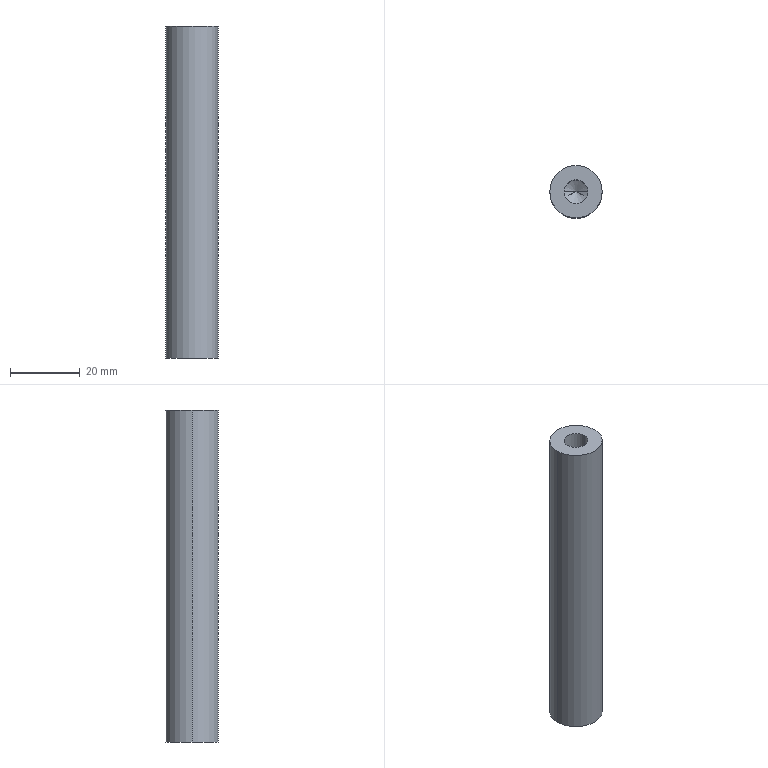Part | STEP file | Cuon T phu H01_10_1 | 1 solid | 8 faces | box 15 x 15 x 95 mm | volume 16046 mm3 | cylinder 4 | cone 2 | plane 2 | commonest cylinder face diameters 6.8 x2 15 x2
STEP:
#1=CARTESIAN_POINT('',(0.,0.,0.));
#2=DIRECTION('',(0.,0.,1.));
#3=DIRECTION('',(1.,0.,0.));
#4=AXIS2_PLACEMENT_3D('',#1,#2,#3);
#5=CARTESIAN_POINT('',(3.4,0.,27.75));
#6=VERTEX_POINT('',#5);
#7=CARTESIAN_POINT('',(3.4,0.,47.5));
#8=VERTEX_POINT('',#7);
#9=CARTESIAN_POINT('',(3.4,0.,47.5));
#10=DIRECTION('',(0.,0.,1.));
#11=VECTOR('',#10,1.);
#12=LINE('',#9,#11);
#13=CARTESIAN_POINT('',(0.,0.,47.5));
#14=DIRECTION('',(0.,0.,1.));
#15=DIRECTION('',(1.,0.,0.));
#16=AXIS2_PLACEMENT_3D('',#13,#14,#15);
#17=CYLINDRICAL_SURFACE('',#16,3.4);
#18=CARTESIAN_POINT('',(6.283,0.));
#19=DIRECTION('',(0.,1.));
#20=VECTOR('',#19,1.);
#21=LINE('',#18,#20);
#22=(GEOMETRIC_REPRESENTATION_CONTEXT(2)PARAMETRIC_REPRESENTATION_CONTEXT()REPRESENTATION_CONTEXT('',''));
#23=DEFINITIONAL_REPRESENTATION('',(#21),#22);
#24=PCURVE('',#17,#23);
#25=CARTESIAN_POINT('',(0.,0.,47.5));
#26=DIRECTION('',(0.,0.,1.));
#27=DIRECTION('',(1.,0.,0.));
#28=AXIS2_PLACEMENT_3D('',#25,#26,#27);
#29=CYLINDRICAL_SURFACE('',#28,3.4);
#30=CARTESIAN_POINT('',(0.,0.));
#31=DIRECTION('',(0.,1.));
#32=VECTOR('',#31,1.);
#33=LINE('',#30,#32);
#34=(GEOMETRIC_REPRESENTATION_CONTEXT(2)PARAMETRIC_REPRESENTATION_CONTEXT()REPRESENTATION_CONTEXT('',''));
#35=DEFINITIONAL_REPRESENTATION('',(#33),#34);
#36=PCURVE('',#29,#35);
#37=SURFACE_CURVE('',#12,(#24,#36),.PCURVE_S1.);
#38=EDGE_CURVE('',#6,#8,#37,.T.);
#39=ORIENTED_EDGE('',*,*,#38,.T.);
#40=CARTESIAN_POINT('',(-3.4,0.,47.5));
#41=VERTEX_POINT('',#40);
#42=CARTESIAN_POINT('',(0.,0.,47.5));
#43=DIRECTION('',(0.,0.,1.));
#44=DIRECTION('',(1.,0.,0.));
#45=AXIS2_PLACEMENT_3D('',#42,#43,#44);
#46=CIRCLE('',#45,3.4);
#47=CARTESIAN_POINT('',(0.,0.));
#48=DIRECTION('',(1.,0.));
#49=VECTOR('',#48,1.);
#50=LINE('',#47,#49);
#51=(GEOMETRIC_REPRESENTATION_CONTEXT(2)PARAMETRIC_REPRESENTATION_CONTEXT()REPRESENTATION_CONTEXT('',''));
#52=DEFINITIONAL_REPRESENTATION('',(#50),#51);
#53=PCURVE('',#17,#52);
#54=CARTESIAN_POINT('',(0.,0.,47.5));
#55=DIRECTION('',(0.,0.,1.));
#56=DIRECTION('',(1.,0.,0.));
#57=AXIS2_PLACEMENT_3D('',#54,#55,#56);
#58=PLANE('',#57);
#59=CARTESIAN_POINT('',(0.,0.));
#60=DIRECTION('',(1.,0.));
#61=AXIS2_PLACEMENT_2D('',#59,#60);
#62=CIRCLE('',#61,3.4);
#63=(GEOMETRIC_REPRESENTATION_CONTEXT(2)PARAMETRIC_REPRESENTATION_CONTEXT()REPRESENTATION_CONTEXT('',''));
#64=DEFINITIONAL_REPRESENTATION('',(#62),#63);
#65=PCURVE('',#58,#64);
#66=SURFACE_CURVE('',#46,(#53,#65),.PCURVE_S1.);
#67=EDGE_CURVE('',#41,#8,#66,.T.);
#68=ORIENTED_EDGE('',*,*,#67,.F.);
#69=CARTESIAN_POINT('',(-3.4,0.,27.75));
#70=VERTEX_POINT('',#69);
#71=CARTESIAN_POINT('',(-3.4,0.,47.5));
#72=DIRECTION('',(0.,0.,1.));
#73=VECTOR('',#72,1.);
#74=LINE('',#71,#73);
#75=CARTESIAN_POINT('',(3.142,0.));
#76=DIRECTION('',(0.,1.));
#77=VECTOR('',#76,1.);
#78=LINE('',#75,#77);
#79=(GEOMETRIC_REPRESENTATION_CONTEXT(2)PARAMETRIC_REPRESENTATION_CONTEXT()REPRESENTATION_CONTEXT('',''));
#80=DEFINITIONAL_REPRESENTATION('',(#78),#79);
#81=PCURVE('',#17,#80);
#82=CARTESIAN_POINT('',(3.142,0.));
#83=DIRECTION('',(0.,1.));
#84=VECTOR('',#83,1.);
#85=LINE('',#82,#84);
#86=(GEOMETRIC_REPRESENTATION_CONTEXT(2)PARAMETRIC_REPRESENTATION_CONTEXT()REPRESENTATION_CONTEXT('',''));
#87=DEFINITIONAL_REPRESENTATION('',(#85),#86);
#88=PCURVE('',#29,#87);
#89=SURFACE_CURVE('',#74,(#81,#88),.PCURVE_S1.);
#90=EDGE_CURVE('',#70,#41,#89,.T.);
#91=ORIENTED_EDGE('',*,*,#90,.F.);
#92=CARTESIAN_POINT('',(0.,0.,27.75));
#93=DIRECTION('',(0.,0.,1.));
#94=DIRECTION('',(1.,0.,0.));
#95=AXIS2_PLACEMENT_3D('',#92,#93,#94);
#96=CIRCLE('',#95,3.4);
#97=CARTESIAN_POINT('',(0.,-19.75));
#98=DIRECTION('',(1.,0.));
#99=VECTOR('',#98,1.);
#100=LINE('',#97,#99);
#101=(GEOMETRIC_REPRESENTATION_CONTEXT(2)PARAMETRIC_REPRESENTATION_CONTEXT()REPRESENTATION_CONTEXT('',''));
#102=DEFINITIONAL_REPRESENTATION('',(#100),#101);
#103=PCURVE('',#17,#102);
#104=CARTESIAN_POINT('',(0.,0.,27.75));
#105=DIRECTION('',(0.,0.,1.));
#106=DIRECTION('',(1.,0.,0.));
#107=AXIS2_PLACEMENT_3D('',#104,#105,#106);
#108=CONICAL_SURFACE('',#107,3.4,1.03);
#109=CARTESIAN_POINT('',(0.,0.));
#110=DIRECTION('',(1.,0.));
#111=VECTOR('',#110,1.);
#112=LINE('',#109,#111);
#113=(GEOMETRIC_REPRESENTATION_CONTEXT(2)PARAMETRIC_REPRESENTATION_CONTEXT()REPRESENTATION_CONTEXT('',''));
#114=DEFINITIONAL_REPRESENTATION('',(#112),#113);
#115=PCURVE('',#108,#114);
#116=SURFACE_CURVE('',#96,(#103,#115),.PCURVE_S1.);
#117=EDGE_CURVE('',#70,#6,#116,.T.);
#118=ORIENTED_EDGE('',*,*,#117,.T.);
#119=EDGE_LOOP('',(#39,#68,#91,#118));
#120=FACE_BOUND('',#119,.F.);
#121=ADVANCED_FACE('',(#120),#17,.F.);
#122=ORIENTED_EDGE('',*,*,#117,.F.);
#123=CARTESIAN_POINT('',(0.,0.,25.707));
#124=VERTEX_POINT('',#123);
#125=CARTESIAN_POINT('',(-3.4,0.,27.75));
#126=DIRECTION('',(-0.8572,0.,0.515));
#127=VECTOR('',#126,1.);
#128=LINE('',#125,#127);
#129=CARTESIAN_POINT('',(3.142,0.));
#130=DIRECTION('',(0.,1.));
#131=VECTOR('',#130,1.);
#132=LINE('',#129,#131);
#133=(GEOMETRIC_REPRESENTATION_CONTEXT(2)PARAMETRIC_REPRESENTATION_CONTEXT()REPRESENTATION_CONTEXT('',''));
#134=DEFINITIONAL_REPRESENTATION('',(#132),#133);
#135=PCURVE('',#108,#134);
#136=CARTESIAN_POINT('',(0.,0.,27.75));
#137=DIRECTION('',(0.,0.,1.));
#138=DIRECTION('',(1.,0.,0.));
#139=AXIS2_PLACEMENT_3D('',#136,#137,#138);
#140=CONICAL_SURFACE('',#139,3.4,1.03);
#141=CARTESIAN_POINT('',(3.142,0.));
#142=DIRECTION('',(0.,1.));
#143=VECTOR('',#142,1.);
#144=LINE('',#141,#143);
#145=(GEOMETRIC_REPRESENTATION_CONTEXT(2)PARAMETRIC_REPRESENTATION_CONTEXT()REPRESENTATION_CONTEXT('',''));
#146=DEFINITIONAL_REPRESENTATION('',(#144),#145);
#147=PCURVE('',#140,#146);
#148=SURFACE_CURVE('',#128,(#135,#147),.PCURVE_S1.);
#149=EDGE_CURVE('',#124,#70,#148,.T.);
#150=ORIENTED_EDGE('',*,*,#149,.F.);
#151=CARTESIAN_POINT('',(3.4,0.,27.75));
#152=DIRECTION('',(0.8572,0.,0.515));
#153=VECTOR('',#152,1.);
#154=LINE('',#151,#153);
#155=CARTESIAN_POINT('',(6.283,0.));
#156=DIRECTION('',(0.,1.));
#157=VECTOR('',#156,1.);
#158=LINE('',#155,#157);
#159=(GEOMETRIC_REPRESENTATION_CONTEXT(2)PARAMETRIC_REPRESENTATION_CONTEXT()REPRESENTATION_CONTEXT('',''));
#160=DEFINITIONAL_REPRESENTATION('',(#158),#159);
#161=PCURVE('',#108,#160);
#162=CARTESIAN_POINT('',(0.,0.));
#163=DIRECTION('',(0.,1.));
#164=VECTOR('',#163,1.);
#165=LINE('',#162,#164);
#166=(GEOMETRIC_REPRESENTATION_CONTEXT(2)PARAMETRIC_REPRESENTATION_CONTEXT()REPRESENTATION_CONTEXT('',''));
#167=DEFINITIONAL_REPRESENTATION('',(#165),#166);
#168=PCURVE('',#140,#167);
#169=SURFACE_CURVE('',#154,(#161,#168),.PCURVE_S1.);
#170=EDGE_CURVE('',#124,#6,#169,.T.);
#171=ORIENTED_EDGE('',*,*,#170,.T.);
#172=EDGE_LOOP('',(#122,#150,#171));
#173=FACE_BOUND('',#172,.F.);
#174=ADVANCED_FACE('',(#173),#108,.F.);
#175=CARTESIAN_POINT('',(7.5,0.,47.5));
#176=VERTEX_POINT('',#175);
#177=CARTESIAN_POINT('',(-7.5,0.,47.5));
#178=VERTEX_POINT('',#177);
#179=CARTESIAN_POINT('',(0.,0.,47.5));
#180=DIRECTION('',(0.,0.,1.));
#181=DIRECTION('',(1.,0.,0.));
#182=AXIS2_PLACEMENT_3D('',#179,#180,#181);
#183=CIRCLE('',#182,7.5);
#184=CARTESIAN_POINT('',(0.,0.,47.5));
#185=DIRECTION('',(0.,0.,-1.));
#186=DIRECTION('',(-1.,0.,0.));
#187=AXIS2_PLACEMENT_3D('',#184,#185,#186);
#188=CYLINDRICAL_SURFACE('',#187,7.5);
#189=CARTESIAN_POINT('',(3.142,0.));
#190=DIRECTION('',(-1.,0.));
#191=VECTOR('',#190,1.);
#192=LINE('',#189,#191);
#193=(GEOMETRIC_REPRESENTATION_CONTEXT(2)PARAMETRIC_REPRESENTATION_CONTEXT()REPRESENTATION_CONTEXT('',''));
#194=DEFINITIONAL_REPRESENTATION('',(#192),#193);
#195=PCURVE('',#188,#194);
#196=CARTESIAN_POINT('',(0.,0.));
#197=DIRECTION('',(1.,0.));
#198=AXIS2_PLACEMENT_2D('',#196,#197);
#199=CIRCLE('',#198,7.5);
#200=(GEOMETRIC_REPRESENTATION_CONTEXT(2)PARAMETRIC_REPRESENTATION_CONTEXT()REPRESENTATION_CONTEXT('',''));
#201=DEFINITIONAL_REPRESENTATION('',(#199),#200);
#202=PCURVE('',#58,#201);
#203=SURFACE_CURVE('',#183,(#195,#202),.PCURVE_S1.);
#204=EDGE_CURVE('',#176,#178,#203,.T.);
#205=ORIENTED_EDGE('',*,*,#204,.F.);
#206=CARTESIAN_POINT('',(7.5,0.,-47.5));
#207=VERTEX_POINT('',#206);
#208=CARTESIAN_POINT('',(7.5,0.,47.5));
#209=DIRECTION('',(0.,0.,-1.));
#210=VECTOR('',#209,1.);
#211=LINE('',#208,#210);
#212=CARTESIAN_POINT('',(3.142,0.));
#213=DIRECTION('',(0.,1.));
#214=VECTOR('',#213,1.);
#215=LINE('',#212,#214);
#216=(GEOMETRIC_REPRESENTATION_CONTEXT(2)PARAMETRIC_REPRESENTATION_CONTEXT()REPRESENTATION_CONTEXT('',''));
#217=DEFINITIONAL_REPRESENTATION('',(#215),#216);
#218=PCURVE('',#188,#217);
#219=CARTESIAN_POINT('',(0.,0.,47.5));
#220=DIRECTION('',(0.,0.,-1.));
#221=DIRECTION('',(-1.,0.,0.));
#222=AXIS2_PLACEMENT_3D('',#219,#220,#221);
#223=CYLINDRICAL_SURFACE('',#222,7.5);
#224=CARTESIAN_POINT('',(3.142,0.));
#225=DIRECTION('',(0.,1.));
#226=VECTOR('',#225,1.);
#227=LINE('',#224,#226);
#228=(GEOMETRIC_REPRESENTATION_CONTEXT(2)PARAMETRIC_REPRESENTATION_CONTEXT()REPRESENTATION_CONTEXT('',''));
#229=DEFINITIONAL_REPRESENTATION('',(#227),#228);
#230=PCURVE('',#223,#229);
#231=SURFACE_CURVE('',#211,(#218,#230),.PCURVE_S1.);
#232=EDGE_CURVE('',#176,#207,#231,.T.);
#233=ORIENTED_EDGE('',*,*,#232,.T.);
#234=CARTESIAN_POINT('',(-7.5,0.,-47.5));
#235=VERTEX_POINT('',#234);
#236=CARTESIAN_POINT('',(0.,0.,-47.5));
#237=DIRECTION('',(0.,0.,1.));
#238=DIRECTION('',(1.,0.,0.));
#239=AXIS2_PLACEMENT_3D('',#236,#237,#238);
#240=CIRCLE('',#239,7.5);
#241=CARTESIAN_POINT('',(3.142,95.));
#242=DIRECTION('',(-1.,0.));
#243=VECTOR('',#242,1.);
#244=LINE('',#241,#243);
#245=(GEOMETRIC_REPRESENTATION_CONTEXT(2)PARAMETRIC_REPRESENTATION_CONTEXT()REPRESENTATION_CONTEXT('',''));
#246=DEFINITIONAL_REPRESENTATION('',(#244),#245);
#247=PCURVE('',#188,#246);
#248=CARTESIAN_POINT('',(0.,0.,-47.5));
#249=DIRECTION('',(0.,0.,1.));
#250=DIRECTION('',(1.,0.,0.));
#251=AXIS2_PLACEMENT_3D('',#248,#249,#250);
#252=PLANE('',#251);
#253=CARTESIAN_POINT('',(0.,0.));
#254=DIRECTION('',(1.,0.));
#255=AXIS2_PLACEMENT_2D('',#253,#254);
#256=CIRCLE('',#255,7.5);
#257=(GEOMETRIC_REPRESENTATION_CONTEXT(2)PARAMETRIC_REPRESENTATION_CONTEXT()REPRESENTATION_CONTEXT('',''));
#258=DEFINITIONAL_REPRESENTATION('',(#256),#257);
#259=PCURVE('',#252,#258);
#260=SURFACE_CURVE('',#240,(#247,#259),.PCURVE_S1.);
#261=EDGE_CURVE('',#207,#235,#260,.T.);
#262=ORIENTED_EDGE('',*,*,#261,.T.);
#263=CARTESIAN_POINT('',(-7.5,0.,47.5));
#264=DIRECTION('',(0.,0.,-1.));
#265=VECTOR('',#264,1.);
#266=LINE('',#263,#265);
#267=CARTESIAN_POINT('',(0.,0.));
#268=DIRECTION('',(0.,1.));
#269=VECTOR('',#268,1.);
#270=LINE('',#267,#269);
#271=(GEOMETRIC_REPRESENTATION_CONTEXT(2)PARAMETRIC_REPRESENTATION_CONTEXT()REPRESENTATION_CONTEXT('',''));
#272=DEFINITIONAL_REPRESENTATION('',(#270),#271);
#273=PCURVE('',#188,#272);
#274=CARTESIAN_POINT('',(6.283,0.));
#275=DIRECTION('',(0.,1.));
#276=VECTOR('',#275,1.);
#277=LINE('',#274,#276);
#278=(GEOMETRIC_REPRESENTATION_CONTEXT(2)PARAMETRIC_REPRESENTATION_CONTEXT()REPRESENTATION_CONTEXT('',''));
#279=DEFINITIONAL_REPRESENTATION('',(#277),#278);
#280=PCURVE('',#223,#279);
#281=SURFACE_CURVE('',#266,(#273,#280),.PCURVE_S1.);
#282=EDGE_CURVE('',#178,#235,#281,.T.);
#283=ORIENTED_EDGE('',*,*,#282,.F.);
#284=EDGE_LOOP('',(#205,#233,#262,#283));
#285=FACE_BOUND('',#284,.T.);
#286=ADVANCED_FACE('',(#285),#188,.T.);
#287=ORIENTED_EDGE('',*,*,#232,.F.);
#288=CARTESIAN_POINT('',(0.,0.,47.5));
#289=DIRECTION('',(0.,0.,1.));
#290=DIRECTION('',(1.,0.,0.));
#291=AXIS2_PLACEMENT_3D('',#288,#289,#290);
#292=CIRCLE('',#291,7.5);
#293=CARTESIAN_POINT('',(9.425,0.));
#294=DIRECTION('',(-1.,0.));
#295=VECTOR('',#294,1.);
#296=LINE('',#293,#295);
#297=(GEOMETRIC_REPRESENTATION_CONTEXT(2)PARAMETRIC_REPRESENTATION_CONTEXT()REPRESENTATION_CONTEXT('',''));
#298=DEFINITIONAL_REPRESENTATION('',(#296),#297);
#299=PCURVE('',#223,#298);
#300=CARTESIAN_POINT('',(0.,0.));
#301=DIRECTION('',(1.,0.));
#302=AXIS2_PLACEMENT_2D('',#300,#301);
#303=CIRCLE('',#302,7.5);
#304=(GEOMETRIC_REPRESENTATION_CONTEXT(2)PARAMETRIC_REPRESENTATION_CONTEXT()REPRESENTATION_CONTEXT('',''));
#305=DEFINITIONAL_REPRESENTATION('',(#303),#304);
#306=PCURVE('',#58,#305);
#307=SURFACE_CURVE('',#292,(#299,#306),.PCURVE_S1.);
#308=EDGE_CURVE('',#178,#176,#307,.T.);
#309=ORIENTED_EDGE('',*,*,#308,.F.);
#310=ORIENTED_EDGE('',*,*,#282,.T.);
#311=CARTESIAN_POINT('',(0.,0.,-47.5));
#312=DIRECTION('',(0.,0.,1.));
#313=DIRECTION('',(1.,0.,0.));
#314=AXIS2_PLACEMENT_3D('',#311,#312,#313);
#315=CIRCLE('',#314,7.5);
#316=CARTESIAN_POINT('',(9.425,95.));
#317=DIRECTION('',(-1.,0.));
#318=VECTOR('',#317,1.);
#319=LINE('',#316,#318);
#320=(GEOMETRIC_REPRESENTATION_CONTEXT(2)PARAMETRIC_REPRESENTATION_CONTEXT()REPRESENTATION_CONTEXT('',''));
#321=DEFINITIONAL_REPRESENTATION('',(#319),#320);
#322=PCURVE('',#223,#321);
#323=CARTESIAN_POINT('',(0.,0.));
#324=DIRECTION('',(1.,0.));
#325=AXIS2_PLACEMENT_2D('',#323,#324);
#326=CIRCLE('',#325,7.5);
#327=(GEOMETRIC_REPRESENTATION_CONTEXT(2)PARAMETRIC_REPRESENTATION_CONTEXT()REPRESENTATION_CONTEXT('',''));
#328=DEFINITIONAL_REPRESENTATION('',(#326),#327);
#329=PCURVE('',#252,#328);
#330=SURFACE_CURVE('',#315,(#322,#329),.PCURVE_S1.);
#331=EDGE_CURVE('',#235,#207,#330,.T.);
#332=ORIENTED_EDGE('',*,*,#331,.T.);
#333=EDGE_LOOP('',(#287,#309,#310,#332));
#334=FACE_BOUND('',#333,.T.);
#335=ADVANCED_FACE('',(#334),#223,.T.);
#336=CARTESIAN_POINT('',(0.,0.,47.5));
#337=DIRECTION('',(0.,0.,1.));
#338=DIRECTION('',(1.,0.,0.));
#339=AXIS2_PLACEMENT_3D('',#336,#337,#338);
#340=CIRCLE('',#339,3.4);
#341=CARTESIAN_POINT('',(0.,0.));
#342=DIRECTION('',(1.,0.));
#343=AXIS2_PLACEMENT_2D('',#341,#342);
#344=CIRCLE('',#343,3.4);
#345=(GEOMETRIC_REPRESENTATION_CONTEXT(2)PARAMETRIC_REPRESENTATION_CONTEXT()REPRESENTATION_CONTEXT('',''));
#346=DEFINITIONAL_REPRESENTATION('',(#344),#345);
#347=PCURVE('',#58,#346);
#348=CARTESIAN_POINT('',(0.,0.));
#349=DIRECTION('',(1.,0.));
#350=VECTOR('',#349,1.);
#351=LINE('',#348,#350);
#352=(GEOMETRIC_REPRESENTATION_CONTEXT(2)PARAMETRIC_REPRESENTATION_CONTEXT()REPRESENTATION_CONTEXT('',''));
#353=DEFINITIONAL_REPRESENTATION('',(#351),#352);
#354=PCURVE('',#29,#353);
#355=SURFACE_CURVE('',#340,(#347,#354),.PCURVE_S1.);
#356=EDGE_CURVE('',#8,#41,#355,.T.);
#357=ORIENTED_EDGE('',*,*,#356,.F.);
#358=ORIENTED_EDGE('',*,*,#67,.F.);
#359=EDGE_LOOP('',(#357,#358));
#360=FACE_BOUND('',#359,.T.);
#361=ORIENTED_EDGE('',*,*,#308,.T.);
#362=ORIENTED_EDGE('',*,*,#204,.T.);
#363=EDGE_LOOP('',(#361,#362));
#364=FACE_BOUND('',#363,.T.);
#365=ADVANCED_FACE('',(#360,#364),#58,.T.);
#366=ORIENTED_EDGE('',*,*,#331,.F.);
#367=ORIENTED_EDGE('',*,*,#261,.F.);
#368=EDGE_LOOP('',(#366,#367));
#369=FACE_BOUND('',#368,.T.);
#370=ADVANCED_FACE('',(#369),#252,.F.);
#371=CARTESIAN_POINT('',(0.,0.,27.75));
#372=DIRECTION('',(0.,0.,1.));
#373=DIRECTION('',(1.,0.,0.));
#374=AXIS2_PLACEMENT_3D('',#371,#372,#373);
#375=CIRCLE('',#374,3.4);
#376=CARTESIAN_POINT('',(0.,0.));
#377=DIRECTION('',(1.,0.));
#378=VECTOR('',#377,1.);
#379=LINE('',#376,#378);
#380=(GEOMETRIC_REPRESENTATION_CONTEXT(2)PARAMETRIC_REPRESENTATION_CONTEXT()REPRESENTATION_CONTEXT('',''));
#381=DEFINITIONAL_REPRESENTATION('',(#379),#380);
#382=PCURVE('',#140,#381);
#383=CARTESIAN_POINT('',(0.,-19.75));
#384=DIRECTION('',(1.,0.));
#385=VECTOR('',#384,1.);
#386=LINE('',#383,#385);
#387=(GEOMETRIC_REPRESENTATION_CONTEXT(2)PARAMETRIC_REPRESENTATION_CONTEXT()REPRESENTATION_CONTEXT('',''));
#388=DEFINITIONAL_REPRESENTATION('',(#386),#387);
#389=PCURVE('',#29,#388);
#390=SURFACE_CURVE('',#375,(#382,#389),.PCURVE_S1.);
#391=EDGE_CURVE('',#6,#70,#390,.T.);
#392=ORIENTED_EDGE('',*,*,#391,.F.);
#393=ORIENTED_EDGE('',*,*,#170,.F.);
#394=ORIENTED_EDGE('',*,*,#149,.T.);
#395=EDGE_LOOP('',(#392,#393,#394));
#396=FACE_BOUND('',#395,.F.);
#397=ADVANCED_FACE('',(#396),#140,.F.);
#398=ORIENTED_EDGE('',*,*,#356,.F.);
#399=ORIENTED_EDGE('',*,*,#38,.F.);
#400=ORIENTED_EDGE('',*,*,#391,.T.);
#401=ORIENTED_EDGE('',*,*,#90,.T.);
#402=EDGE_LOOP('',(#398,#399,#400,#401));
#403=FACE_BOUND('',#402,.F.);
#404=ADVANCED_FACE('',(#403),#29,.F.);
#405=CLOSED_SHELL('',(#121,#174,#286,#335,#365,#370,#397,#404));
#406=MANIFOLD_SOLID_BREP('',#405);
#407=(LENGTH_UNIT()NAMED_UNIT(*)SI_UNIT(.MILLI.,.METRE.));
#408=UNCERTAINTY_MEASURE_WITH_UNIT(LENGTH_MEASURE(0.0000001),#407,'','');
#409=(NAMED_UNIT(*)PLANE_ANGLE_UNIT()SI_UNIT($,.RADIAN.));
#410=(NAMED_UNIT(*)SI_UNIT($,.STERADIAN.)SOLID_ANGLE_UNIT());
#411=(GEOMETRIC_REPRESENTATION_CONTEXT(3)GLOBAL_UNCERTAINTY_ASSIGNED_CONTEXT((#408))GLOBAL_UNIT_ASSIGNED_CONTEXT((#407,#409,#410))REPRESENTATION_CONTEXT('',''));
#412=ADVANCED_BREP_SHAPE_REPRESENTATION('',(#4,#406),#411);